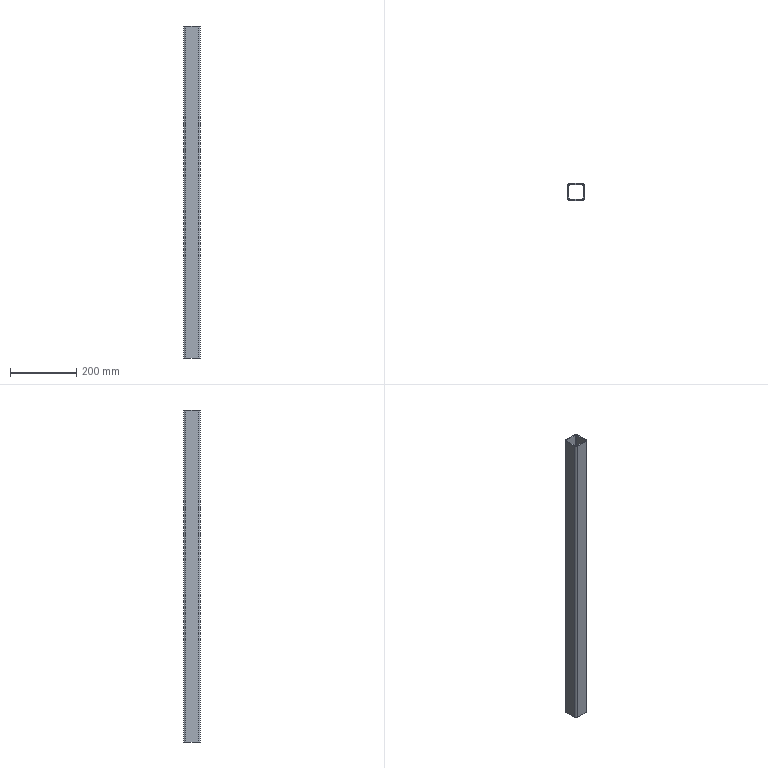Part | SolidWorks | 1 solid | 18 faces | box 50 x 50 x 1000 mm | volume 540823 mm3 | plane 10 | cylinder 8 | commonest cylinder face diameters 6 x4 12 x4
STEP:
#1=CARTESIAN_POINT('',(19.,25.,500.));
#2=VERTEX_POINT('',#1);
#3=CARTESIAN_POINT('',(25.,19.,500.));
#4=VERTEX_POINT('',#3);
#5=CARTESIAN_POINT('',(19.,19.,500.));
#6=DIRECTION('',(0.,0.,-1.));
#7=DIRECTION('',(-1.,0.,0.));
#8=AXIS2_PLACEMENT_3D('',#5,#6,#7);
#9=CIRCLE('',#8,6.);
#10=EDGE_CURVE('',#2,#4,#9,.T.);
#11=ORIENTED_EDGE('',*,*,#10,.T.);
#12=CARTESIAN_POINT('',(25.,19.,-500.));
#13=VERTEX_POINT('',#12);
#14=CARTESIAN_POINT('',(25.,19.,-500.));
#15=DIRECTION('',(0.,0.,1.));
#16=VECTOR('',#15,1000.);
#17=LINE('',#14,#16);
#18=EDGE_CURVE('',#13,#4,#17,.T.);
#19=ORIENTED_EDGE('',*,*,#18,.F.);
#20=CARTESIAN_POINT('',(19.,25.,-500.));
#21=VERTEX_POINT('',#20);
#22=CARTESIAN_POINT('',(19.,19.,-500.));
#23=DIRECTION('',(0.,0.,-1.));
#24=DIRECTION('',(-1.,0.,0.));
#25=AXIS2_PLACEMENT_3D('',#22,#23,#24);
#26=CIRCLE('',#25,6.);
#27=EDGE_CURVE('',#21,#13,#26,.T.);
#28=ORIENTED_EDGE('',*,*,#27,.F.);
#29=CARTESIAN_POINT('',(19.,25.,-500.));
#30=DIRECTION('',(0.,0.,1.));
#31=VECTOR('',#30,1000.);
#32=LINE('',#29,#31);
#33=EDGE_CURVE('',#21,#2,#32,.T.);
#34=ORIENTED_EDGE('',*,*,#33,.T.);
#35=EDGE_LOOP('',(#11,#19,#28,#34));
#36=FACE_OUTER_BOUND('',#35,.T.);
#37=CARTESIAN_POINT('',(19.,19.,-500.));
#38=DIRECTION('',(0.,0.,1.));
#39=DIRECTION('',(1.,0.,0.));
#40=AXIS2_PLACEMENT_3D('',#37,#38,#39);
#41=CYLINDRICAL_SURFACE('',#40,6.);
#42=ADVANCED_FACE('',(#36),#41,.T.);
#43=CARTESIAN_POINT('',(25.,-19.,500.));
#44=VERTEX_POINT('',#43);
#45=CARTESIAN_POINT('',(25.,19.,500.));
#46=DIRECTION('',(0.,-1.,0.));
#47=VECTOR('',#46,1000.);
#48=LINE('',#45,#47);
#49=EDGE_CURVE('',#4,#44,#48,.T.);
#50=ORIENTED_EDGE('',*,*,#49,.T.);
#51=CARTESIAN_POINT('',(25.,-19.,-500.));
#52=VERTEX_POINT('',#51);
#53=CARTESIAN_POINT('',(25.,-19.,-500.));
#54=DIRECTION('',(0.,0.,1.));
#55=VECTOR('',#54,1000.);
#56=LINE('',#53,#55);
#57=EDGE_CURVE('',#52,#44,#56,.T.);
#58=ORIENTED_EDGE('',*,*,#57,.F.);
#59=CARTESIAN_POINT('',(25.,19.,-500.));
#60=DIRECTION('',(0.,-1.,0.));
#61=VECTOR('',#60,1000.);
#62=LINE('',#59,#61);
#63=EDGE_CURVE('',#13,#52,#62,.T.);
#64=ORIENTED_EDGE('',*,*,#63,.F.);
#65=ORIENTED_EDGE('',*,*,#18,.T.);
#66=EDGE_LOOP('',(#50,#58,#64,#65));
#67=FACE_OUTER_BOUND('',#66,.T.);
#68=CARTESIAN_POINT('',(25.,19.,-500.));
#69=DIRECTION('',(-1.,0.,0.));
#70=DIRECTION('',(0.,0.,1.));
#71=AXIS2_PLACEMENT_3D('',#68,#69,#70);
#72=PLANE('',#71);
#73=ADVANCED_FACE('',(#67),#72,.F.);
#74=CARTESIAN_POINT('',(19.,-25.,500.));
#75=VERTEX_POINT('',#74);
#76=CARTESIAN_POINT('',(19.,-19.,500.));
#77=DIRECTION('',(0.,0.,-1.));
#78=DIRECTION('',(-1.,0.,0.));
#79=AXIS2_PLACEMENT_3D('',#76,#77,#78);
#80=CIRCLE('',#79,6.);
#81=EDGE_CURVE('',#44,#75,#80,.T.);
#82=ORIENTED_EDGE('',*,*,#81,.T.);
#83=CARTESIAN_POINT('',(19.,-25.,-500.));
#84=VERTEX_POINT('',#83);
#85=CARTESIAN_POINT('',(19.,-25.,-500.));
#86=DIRECTION('',(0.,0.,1.));
#87=VECTOR('',#86,1000.);
#88=LINE('',#85,#87);
#89=EDGE_CURVE('',#84,#75,#88,.T.);
#90=ORIENTED_EDGE('',*,*,#89,.F.);
#91=CARTESIAN_POINT('',(19.,-19.,-500.));
#92=DIRECTION('',(0.,0.,-1.));
#93=DIRECTION('',(-1.,0.,0.));
#94=AXIS2_PLACEMENT_3D('',#91,#92,#93);
#95=CIRCLE('',#94,6.);
#96=EDGE_CURVE('',#52,#84,#95,.T.);
#97=ORIENTED_EDGE('',*,*,#96,.F.);
#98=ORIENTED_EDGE('',*,*,#57,.T.);
#99=EDGE_LOOP('',(#82,#90,#97,#98));
#100=FACE_OUTER_BOUND('',#99,.T.);
#101=CARTESIAN_POINT('',(19.,-19.,-500.));
#102=DIRECTION('',(0.,0.,1.));
#103=DIRECTION('',(1.,0.,0.));
#104=AXIS2_PLACEMENT_3D('',#101,#102,#103);
#105=CYLINDRICAL_SURFACE('',#104,6.);
#106=ADVANCED_FACE('',(#100),#105,.T.);
#107=CARTESIAN_POINT('',(-19.,-25.,500.));
#108=VERTEX_POINT('',#107);
#109=CARTESIAN_POINT('',(-19.,-25.,500.));
#110=DIRECTION('',(-1.,0.,0.));
#111=VECTOR('',#110,1000.);
#112=LINE('',#109,#111);
#113=EDGE_CURVE('',#75,#108,#112,.T.);
#114=ORIENTED_EDGE('',*,*,#113,.T.);
#115=CARTESIAN_POINT('',(-19.,-25.,-500.));
#116=VERTEX_POINT('',#115);
#117=CARTESIAN_POINT('',(-19.,-25.,-500.));
#118=DIRECTION('',(0.,0.,1.));
#119=VECTOR('',#118,1000.);
#120=LINE('',#117,#119);
#121=EDGE_CURVE('',#116,#108,#120,.T.);
#122=ORIENTED_EDGE('',*,*,#121,.F.);
#123=CARTESIAN_POINT('',(-19.,-25.,-500.));
#124=DIRECTION('',(-1.,0.,0.));
#125=VECTOR('',#124,1000.);
#126=LINE('',#123,#125);
#127=EDGE_CURVE('',#84,#116,#126,.T.);
#128=ORIENTED_EDGE('',*,*,#127,.F.);
#129=ORIENTED_EDGE('',*,*,#89,.T.);
#130=EDGE_LOOP('',(#114,#122,#128,#129));
#131=FACE_OUTER_BOUND('',#130,.T.);
#132=CARTESIAN_POINT('',(-19.,-25.,-500.));
#133=DIRECTION('',(0.,1.,0.));
#134=DIRECTION('',(0.,0.,1.));
#135=AXIS2_PLACEMENT_3D('',#132,#133,#134);
#136=PLANE('',#135);
#137=ADVANCED_FACE('',(#131),#136,.F.);
#138=CARTESIAN_POINT('',(-25.,-19.,500.));
#139=VERTEX_POINT('',#138);
#140=CARTESIAN_POINT('',(-19.,-19.,500.));
#141=DIRECTION('',(0.,0.,-1.));
#142=DIRECTION('',(-1.,0.,0.));
#143=AXIS2_PLACEMENT_3D('',#140,#141,#142);
#144=CIRCLE('',#143,6.);
#145=EDGE_CURVE('',#108,#139,#144,.T.);
#146=ORIENTED_EDGE('',*,*,#145,.T.);
#147=CARTESIAN_POINT('',(-25.,-19.,-500.));
#148=VERTEX_POINT('',#147);
#149=CARTESIAN_POINT('',(-25.,-19.,-500.));
#150=DIRECTION('',(0.,0.,1.));
#151=VECTOR('',#150,1000.);
#152=LINE('',#149,#151);
#153=EDGE_CURVE('',#148,#139,#152,.T.);
#154=ORIENTED_EDGE('',*,*,#153,.F.);
#155=CARTESIAN_POINT('',(-19.,-19.,-500.));
#156=DIRECTION('',(0.,0.,-1.));
#157=DIRECTION('',(-1.,0.,0.));
#158=AXIS2_PLACEMENT_3D('',#155,#156,#157);
#159=CIRCLE('',#158,6.);
#160=EDGE_CURVE('',#116,#148,#159,.T.);
#161=ORIENTED_EDGE('',*,*,#160,.F.);
#162=ORIENTED_EDGE('',*,*,#121,.T.);
#163=EDGE_LOOP('',(#146,#154,#161,#162));
#164=FACE_OUTER_BOUND('',#163,.T.);
#165=CARTESIAN_POINT('',(-19.,-19.,-500.));
#166=DIRECTION('',(0.,0.,1.));
#167=DIRECTION('',(1.,0.,0.));
#168=AXIS2_PLACEMENT_3D('',#165,#166,#167);
#169=CYLINDRICAL_SURFACE('',#168,6.);
#170=ADVANCED_FACE('',(#164),#169,.T.);
#171=CARTESIAN_POINT('',(-25.,19.,500.));
#172=VERTEX_POINT('',#171);
#173=CARTESIAN_POINT('',(-25.,-19.,500.));
#174=DIRECTION('',(0.,1.,0.));
#175=VECTOR('',#174,1000.);
#176=LINE('',#173,#175);
#177=EDGE_CURVE('',#139,#172,#176,.T.);
#178=ORIENTED_EDGE('',*,*,#177,.T.);
#179=CARTESIAN_POINT('',(-25.,19.,-500.));
#180=VERTEX_POINT('',#179);
#181=CARTESIAN_POINT('',(-25.,19.,-500.));
#182=DIRECTION('',(0.,0.,1.));
#183=VECTOR('',#182,1000.);
#184=LINE('',#181,#183);
#185=EDGE_CURVE('',#180,#172,#184,.T.);
#186=ORIENTED_EDGE('',*,*,#185,.F.);
#187=CARTESIAN_POINT('',(-25.,-19.,-500.));
#188=DIRECTION('',(0.,1.,0.));
#189=VECTOR('',#188,1000.);
#190=LINE('',#187,#189);
#191=EDGE_CURVE('',#148,#180,#190,.T.);
#192=ORIENTED_EDGE('',*,*,#191,.F.);
#193=ORIENTED_EDGE('',*,*,#153,.T.);
#194=EDGE_LOOP('',(#178,#186,#192,#193));
#195=FACE_OUTER_BOUND('',#194,.T.);
#196=CARTESIAN_POINT('',(-25.,-19.,-500.));
#197=DIRECTION('',(1.,0.,0.));
#198=DIRECTION('',(0.,0.,-1.));
#199=AXIS2_PLACEMENT_3D('',#196,#197,#198);
#200=PLANE('',#199);
#201=ADVANCED_FACE('',(#195),#200,.F.);
#202=CARTESIAN_POINT('',(-19.,25.,500.));
#203=VERTEX_POINT('',#202);
#204=CARTESIAN_POINT('',(-19.,19.,500.));
#205=DIRECTION('',(0.,0.,-1.));
#206=DIRECTION('',(-1.,0.,0.));
#207=AXIS2_PLACEMENT_3D('',#204,#205,#206);
#208=CIRCLE('',#207,6.);
#209=EDGE_CURVE('',#172,#203,#208,.T.);
#210=ORIENTED_EDGE('',*,*,#209,.T.);
#211=CARTESIAN_POINT('',(-19.,25.,-500.));
#212=VERTEX_POINT('',#211);
#213=CARTESIAN_POINT('',(-19.,25.,-500.));
#214=DIRECTION('',(0.,0.,1.));
#215=VECTOR('',#214,1000.);
#216=LINE('',#213,#215);
#217=EDGE_CURVE('',#212,#203,#216,.T.);
#218=ORIENTED_EDGE('',*,*,#217,.F.);
#219=CARTESIAN_POINT('',(-19.,19.,-500.));
#220=DIRECTION('',(0.,0.,-1.));
#221=DIRECTION('',(-1.,0.,0.));
#222=AXIS2_PLACEMENT_3D('',#219,#220,#221);
#223=CIRCLE('',#222,6.);
#224=EDGE_CURVE('',#180,#212,#223,.T.);
#225=ORIENTED_EDGE('',*,*,#224,.F.);
#226=ORIENTED_EDGE('',*,*,#185,.T.);
#227=EDGE_LOOP('',(#210,#218,#225,#226));
#228=FACE_OUTER_BOUND('',#227,.T.);
#229=CARTESIAN_POINT('',(-19.,19.,-500.));
#230=DIRECTION('',(0.,0.,1.));
#231=DIRECTION('',(1.,0.,0.));
#232=AXIS2_PLACEMENT_3D('',#229,#230,#231);
#233=CYLINDRICAL_SURFACE('',#232,6.);
#234=ADVANCED_FACE('',(#228),#233,.T.);
#235=CARTESIAN_POINT('',(22.,-19.,500.));
#236=VERTEX_POINT('',#235);
#237=CARTESIAN_POINT('',(19.,-22.,500.));
#238=VERTEX_POINT('',#237);
#239=CARTESIAN_POINT('',(19.,-19.,500.));
#240=DIRECTION('',(0.,0.,-1.));
#241=DIRECTION('',(-1.,0.,0.));
#242=AXIS2_PLACEMENT_3D('',#239,#240,#241);
#243=CIRCLE('',#242,3.);
#244=EDGE_CURVE('',#236,#238,#243,.T.);
#245=ORIENTED_EDGE('',*,*,#244,.F.);
#246=CARTESIAN_POINT('',(22.,-19.,-500.));
#247=VERTEX_POINT('',#246);
#248=CARTESIAN_POINT('',(22.,-19.,-500.));
#249=DIRECTION('',(0.,0.,1.));
#250=VECTOR('',#249,1000.);
#251=LINE('',#248,#250);
#252=EDGE_CURVE('',#247,#236,#251,.T.);
#253=ORIENTED_EDGE('',*,*,#252,.F.);
#254=CARTESIAN_POINT('',(19.,-22.,-500.));
#255=VERTEX_POINT('',#254);
#256=CARTESIAN_POINT('',(19.,-19.,-500.));
#257=DIRECTION('',(0.,0.,-1.));
#258=DIRECTION('',(-1.,0.,0.));
#259=AXIS2_PLACEMENT_3D('',#256,#257,#258);
#260=CIRCLE('',#259,3.);
#261=EDGE_CURVE('',#247,#255,#260,.T.);
#262=ORIENTED_EDGE('',*,*,#261,.T.);
#263=CARTESIAN_POINT('',(19.,-22.,-500.));
#264=DIRECTION('',(0.,0.,1.));
#265=VECTOR('',#264,1000.);
#266=LINE('',#263,#265);
#267=EDGE_CURVE('',#255,#238,#266,.T.);
#268=ORIENTED_EDGE('',*,*,#267,.T.);
#269=EDGE_LOOP('',(#245,#253,#262,#268));
#270=FACE_OUTER_BOUND('',#269,.T.);
#271=CARTESIAN_POINT('',(19.,-19.,-500.));
#272=DIRECTION('',(0.,0.,1.));
#273=DIRECTION('',(1.,0.,0.));
#274=AXIS2_PLACEMENT_3D('',#271,#272,#273);
#275=CYLINDRICAL_SURFACE('',#274,3.);
#276=ADVANCED_FACE('',(#270),#275,.F.);
#277=CARTESIAN_POINT('',(22.,19.,500.));
#278=VERTEX_POINT('',#277);
#279=CARTESIAN_POINT('',(22.,19.,500.));
#280=DIRECTION('',(0.,-1.,0.));
#281=VECTOR('',#280,1000.);
#282=LINE('',#279,#281);
#283=EDGE_CURVE('',#278,#236,#282,.T.);
#284=ORIENTED_EDGE('',*,*,#283,.F.);
#285=CARTESIAN_POINT('',(22.,19.,-500.));
#286=VERTEX_POINT('',#285);
#287=CARTESIAN_POINT('',(22.,19.,-500.));
#288=DIRECTION('',(0.,0.,1.));
#289=VECTOR('',#288,1000.);
#290=LINE('',#287,#289);
#291=EDGE_CURVE('',#286,#278,#290,.T.);
#292=ORIENTED_EDGE('',*,*,#291,.F.);
#293=CARTESIAN_POINT('',(22.,19.,-500.));
#294=DIRECTION('',(0.,-1.,0.));
#295=VECTOR('',#294,1000.);
#296=LINE('',#293,#295);
#297=EDGE_CURVE('',#286,#247,#296,.T.);
#298=ORIENTED_EDGE('',*,*,#297,.T.);
#299=ORIENTED_EDGE('',*,*,#252,.T.);
#300=EDGE_LOOP('',(#284,#292,#298,#299));
#301=FACE_OUTER_BOUND('',#300,.T.);
#302=CARTESIAN_POINT('',(22.,19.,-500.));
#303=DIRECTION('',(-1.,0.,0.));
#304=DIRECTION('',(0.,0.,1.));
#305=AXIS2_PLACEMENT_3D('',#302,#303,#304);
#306=PLANE('',#305);
#307=ADVANCED_FACE('',(#301),#306,.T.);
#308=CARTESIAN_POINT('',(19.,22.,500.));
#309=VERTEX_POINT('',#308);
#310=CARTESIAN_POINT('',(19.,19.,500.));
#311=DIRECTION('',(0.,0.,-1.));
#312=DIRECTION('',(-1.,0.,0.));
#313=AXIS2_PLACEMENT_3D('',#310,#311,#312);
#314=CIRCLE('',#313,3.);
#315=EDGE_CURVE('',#309,#278,#314,.T.);
#316=ORIENTED_EDGE('',*,*,#315,.F.);
#317=CARTESIAN_POINT('',(19.,22.,-500.));
#318=VERTEX_POINT('',#317);
#319=CARTESIAN_POINT('',(19.,22.,-500.));
#320=DIRECTION('',(0.,0.,1.));
#321=VECTOR('',#320,1000.);
#322=LINE('',#319,#321);
#323=EDGE_CURVE('',#318,#309,#322,.T.);
#324=ORIENTED_EDGE('',*,*,#323,.F.);
#325=CARTESIAN_POINT('',(19.,19.,-500.));
#326=DIRECTION('',(0.,0.,-1.));
#327=DIRECTION('',(-1.,0.,0.));
#328=AXIS2_PLACEMENT_3D('',#325,#326,#327);
#329=CIRCLE('',#328,3.);
#330=EDGE_CURVE('',#318,#286,#329,.T.);
#331=ORIENTED_EDGE('',*,*,#330,.T.);
#332=ORIENTED_EDGE('',*,*,#291,.T.);
#333=EDGE_LOOP('',(#316,#324,#331,#332));
#334=FACE_OUTER_BOUND('',#333,.T.);
#335=CARTESIAN_POINT('',(19.,19.,-500.));
#336=DIRECTION('',(0.,0.,1.));
#337=DIRECTION('',(1.,0.,0.));
#338=AXIS2_PLACEMENT_3D('',#335,#336,#337);
#339=CYLINDRICAL_SURFACE('',#338,3.);
#340=ADVANCED_FACE('',(#334),#339,.F.);
#341=CARTESIAN_POINT('',(-19.,22.,500.));
#342=VERTEX_POINT('',#341);
#343=CARTESIAN_POINT('',(19.,22.,500.));
#344=DIRECTION('',(1.,0.,0.));
#345=VECTOR('',#344,1000.);
#346=LINE('',#343,#345);
#347=EDGE_CURVE('',#342,#309,#346,.T.);
#348=ORIENTED_EDGE('',*,*,#347,.F.);
#349=CARTESIAN_POINT('',(-19.,22.,-500.));
#350=VERTEX_POINT('',#349);
#351=CARTESIAN_POINT('',(-19.,22.,-500.));
#352=DIRECTION('',(0.,0.,1.));
#353=VECTOR('',#352,1000.);
#354=LINE('',#351,#353);
#355=EDGE_CURVE('',#350,#342,#354,.T.);
#356=ORIENTED_EDGE('',*,*,#355,.F.);
#357=CARTESIAN_POINT('',(19.,22.,-500.));
#358=DIRECTION('',(1.,0.,0.));
#359=VECTOR('',#358,1000.);
#360=LINE('',#357,#359);
#361=EDGE_CURVE('',#350,#318,#360,.T.);
#362=ORIENTED_EDGE('',*,*,#361,.T.);
#363=ORIENTED_EDGE('',*,*,#323,.T.);
#364=EDGE_LOOP('',(#348,#356,#362,#363));
#365=FACE_OUTER_BOUND('',#364,.T.);
#366=CARTESIAN_POINT('',(19.,22.,-500.));
#367=DIRECTION('',(0.,-1.,0.));
#368=DIRECTION('',(0.,0.,-1.));
#369=AXIS2_PLACEMENT_3D('',#366,#367,#368);
#370=PLANE('',#369);
#371=ADVANCED_FACE('',(#365),#370,.T.);
#372=CARTESIAN_POINT('',(-22.,19.,500.));
#373=VERTEX_POINT('',#372);
#374=CARTESIAN_POINT('',(-19.,19.,500.));
#375=DIRECTION('',(0.,0.,-1.));
#376=DIRECTION('',(-1.,0.,0.));
#377=AXIS2_PLACEMENT_3D('',#374,#375,#376);
#378=CIRCLE('',#377,3.);
#379=EDGE_CURVE('',#373,#342,#378,.T.);
#380=ORIENTED_EDGE('',*,*,#379,.F.);
#381=CARTESIAN_POINT('',(-22.,19.,-500.));
#382=VERTEX_POINT('',#381);
#383=CARTESIAN_POINT('',(-22.,19.,-500.));
#384=DIRECTION('',(0.,0.,1.));
#385=VECTOR('',#384,1000.);
#386=LINE('',#383,#385);
#387=EDGE_CURVE('',#382,#373,#386,.T.);
#388=ORIENTED_EDGE('',*,*,#387,.F.);
#389=CARTESIAN_POINT('',(-19.,19.,-500.));
#390=DIRECTION('',(0.,0.,-1.));
#391=DIRECTION('',(-1.,0.,0.));
#392=AXIS2_PLACEMENT_3D('',#389,#390,#391);
#393=CIRCLE('',#392,3.);
#394=EDGE_CURVE('',#382,#350,#393,.T.);
#395=ORIENTED_EDGE('',*,*,#394,.T.);
#396=ORIENTED_EDGE('',*,*,#355,.T.);
#397=EDGE_LOOP('',(#380,#388,#395,#396));
#398=FACE_OUTER_BOUND('',#397,.T.);
#399=CARTESIAN_POINT('',(-19.,19.,-500.));
#400=DIRECTION('',(0.,0.,1.));
#401=DIRECTION('',(1.,0.,0.));
#402=AXIS2_PLACEMENT_3D('',#399,#400,#401);
#403=CYLINDRICAL_SURFACE('',#402,3.);
#404=ADVANCED_FACE('',(#398),#403,.F.);
#405=CARTESIAN_POINT('',(-22.,-19.,500.));
#406=VERTEX_POINT('',#405);
#407=CARTESIAN_POINT('',(-22.,-19.,500.));
#408=DIRECTION('',(0.,1.,0.));
#409=VECTOR('',#408,1000.);
#410=LINE('',#407,#409);
#411=EDGE_CURVE('',#406,#373,#410,.T.);
#412=ORIENTED_EDGE('',*,*,#411,.F.);
#413=CARTESIAN_POINT('',(-22.,-19.,-500.));
#414=VERTEX_POINT('',#413);
#415=CARTESIAN_POINT('',(-22.,-19.,-500.));
#416=DIRECTION('',(0.,0.,1.));
#417=VECTOR('',#416,1000.);
#418=LINE('',#415,#417);
#419=EDGE_CURVE('',#414,#406,#418,.T.);
#420=ORIENTED_EDGE('',*,*,#419,.F.);
#421=CARTESIAN_POINT('',(-22.,-19.,-500.));
#422=DIRECTION('',(0.,1.,0.));
#423=VECTOR('',#422,1000.);
#424=LINE('',#421,#423);
#425=EDGE_CURVE('',#414,#382,#424,.T.);
#426=ORIENTED_EDGE('',*,*,#425,.T.);
#427=ORIENTED_EDGE('',*,*,#387,.T.);
#428=EDGE_LOOP('',(#412,#420,#426,#427));
#429=FACE_OUTER_BOUND('',#428,.T.);
#430=CARTESIAN_POINT('',(-22.,-19.,-500.));
#431=DIRECTION('',(1.,0.,0.));
#432=DIRECTION('',(0.,0.,-1.));
#433=AXIS2_PLACEMENT_3D('',#430,#431,#432);
#434=PLANE('',#433);
#435=ADVANCED_FACE('',(#429),#434,.T.);
#436=CARTESIAN_POINT('',(-19.,-22.,500.));
#437=VERTEX_POINT('',#436);
#438=CARTESIAN_POINT('',(-19.,-19.,500.));
#439=DIRECTION('',(0.,0.,-1.));
#440=DIRECTION('',(-1.,0.,0.));
#441=AXIS2_PLACEMENT_3D('',#438,#439,#440);
#442=CIRCLE('',#441,3.);
#443=EDGE_CURVE('',#437,#406,#442,.T.);
#444=ORIENTED_EDGE('',*,*,#443,.F.);
#445=CARTESIAN_POINT('',(-19.,-22.,-500.));
#446=VERTEX_POINT('',#445);
#447=CARTESIAN_POINT('',(-19.,-22.,-500.));
#448=DIRECTION('',(0.,0.,1.));
#449=VECTOR('',#448,1000.);
#450=LINE('',#447,#449);
#451=EDGE_CURVE('',#446,#437,#450,.T.);
#452=ORIENTED_EDGE('',*,*,#451,.F.);
#453=CARTESIAN_POINT('',(-19.,-19.,-500.));
#454=DIRECTION('',(0.,0.,-1.));
#455=DIRECTION('',(-1.,0.,0.));
#456=AXIS2_PLACEMENT_3D('',#453,#454,#455);
#457=CIRCLE('',#456,3.);
#458=EDGE_CURVE('',#446,#414,#457,.T.);
#459=ORIENTED_EDGE('',*,*,#458,.T.);
#460=ORIENTED_EDGE('',*,*,#419,.T.);
#461=EDGE_LOOP('',(#444,#452,#459,#460));
#462=FACE_OUTER_BOUND('',#461,.T.);
#463=CARTESIAN_POINT('',(-19.,-19.,-500.));
#464=DIRECTION('',(0.,0.,1.));
#465=DIRECTION('',(1.,0.,0.));
#466=AXIS2_PLACEMENT_3D('',#463,#464,#465);
#467=CYLINDRICAL_SURFACE('',#466,3.);
#468=ADVANCED_FACE('',(#462),#467,.F.);
#469=CARTESIAN_POINT('',(-19.,-22.,500.));
#470=DIRECTION('',(-1.,0.,0.));
#471=VECTOR('',#470,1000.);
#472=LINE('',#469,#471);
#473=EDGE_CURVE('',#238,#437,#472,.T.);
#474=ORIENTED_EDGE('',*,*,#473,.F.);
#475=ORIENTED_EDGE('',*,*,#267,.F.);
#476=CARTESIAN_POINT('',(-19.,-22.,-500.));
#477=DIRECTION('',(-1.,0.,0.));
#478=VECTOR('',#477,1000.);
#479=LINE('',#476,#478);
#480=EDGE_CURVE('',#255,#446,#479,.T.);
#481=ORIENTED_EDGE('',*,*,#480,.T.);
#482=ORIENTED_EDGE('',*,*,#451,.T.);
#483=EDGE_LOOP('',(#474,#475,#481,#482));
#484=FACE_OUTER_BOUND('',#483,.T.);
#485=CARTESIAN_POINT('',(-19.,-22.,-500.));
#486=DIRECTION('',(0.,1.,0.));
#487=DIRECTION('',(0.,0.,1.));
#488=AXIS2_PLACEMENT_3D('',#485,#486,#487);
#489=PLANE('',#488);
#490=ADVANCED_FACE('',(#484),#489,.T.);
#491=CARTESIAN_POINT('',(19.,25.,500.));
#492=DIRECTION('',(1.,0.,0.));
#493=VECTOR('',#492,1000.);
#494=LINE('',#491,#493);
#495=EDGE_CURVE('',#203,#2,#494,.T.);
#496=ORIENTED_EDGE('',*,*,#495,.T.);
#497=ORIENTED_EDGE('',*,*,#33,.F.);
#498=CARTESIAN_POINT('',(19.,25.,-500.));
#499=DIRECTION('',(1.,0.,0.));
#500=VECTOR('',#499,1000.);
#501=LINE('',#498,#500);
#502=EDGE_CURVE('',#212,#21,#501,.T.);
#503=ORIENTED_EDGE('',*,*,#502,.F.);
#504=ORIENTED_EDGE('',*,*,#217,.T.);
#505=EDGE_LOOP('',(#496,#497,#503,#504));
#506=FACE_OUTER_BOUND('',#505,.T.);
#507=CARTESIAN_POINT('',(19.,25.,-500.));
#508=DIRECTION('',(0.,-1.,0.));
#509=DIRECTION('',(0.,0.,-1.));
#510=AXIS2_PLACEMENT_3D('',#507,#508,#509);
#511=PLANE('',#510);
#512=ADVANCED_FACE('',(#506),#511,.F.);
#513=ORIENTED_EDGE('',*,*,#261,.F.);
#514=ORIENTED_EDGE('',*,*,#297,.F.);
#515=ORIENTED_EDGE('',*,*,#330,.F.);
#516=ORIENTED_EDGE('',*,*,#361,.F.);
#517=ORIENTED_EDGE('',*,*,#394,.F.);
#518=ORIENTED_EDGE('',*,*,#425,.F.);
#519=ORIENTED_EDGE('',*,*,#458,.F.);
#520=ORIENTED_EDGE('',*,*,#480,.F.);
#521=EDGE_LOOP('',(#513,#514,#515,#516,#517,#518,#519,#520));
#522=FACE_BOUND('',#521,.T.);
#523=ORIENTED_EDGE('',*,*,#27,.T.);
#524=ORIENTED_EDGE('',*,*,#63,.T.);
#525=ORIENTED_EDGE('',*,*,#96,.T.);
#526=ORIENTED_EDGE('',*,*,#127,.T.);
#527=ORIENTED_EDGE('',*,*,#160,.T.);
#528=ORIENTED_EDGE('',*,*,#191,.T.);
#529=ORIENTED_EDGE('',*,*,#224,.T.);
#530=ORIENTED_EDGE('',*,*,#502,.T.);
#531=EDGE_LOOP('',(#523,#524,#525,#526,#527,#528,#529,#530));
#532=FACE_OUTER_BOUND('',#531,.T.);
#533=CARTESIAN_POINT('',(19.,19.,-500.));
#534=DIRECTION('',(0.,0.,-1.));
#535=DIRECTION('',(-1.,0.,0.));
#536=AXIS2_PLACEMENT_3D('',#533,#534,#535);
#537=PLANE('',#536);
#538=ADVANCED_FACE('',(#522,#532),#537,.T.);
#539=ORIENTED_EDGE('',*,*,#244,.T.);
#540=ORIENTED_EDGE('',*,*,#473,.T.);
#541=ORIENTED_EDGE('',*,*,#443,.T.);
#542=ORIENTED_EDGE('',*,*,#411,.T.);
#543=ORIENTED_EDGE('',*,*,#379,.T.);
#544=ORIENTED_EDGE('',*,*,#347,.T.);
#545=ORIENTED_EDGE('',*,*,#315,.T.);
#546=ORIENTED_EDGE('',*,*,#283,.T.);
#547=EDGE_LOOP('',(#539,#540,#541,#542,#543,#544,#545,#546));
#548=FACE_BOUND('',#547,.T.);
#549=ORIENTED_EDGE('',*,*,#10,.F.);
#550=ORIENTED_EDGE('',*,*,#495,.F.);
#551=ORIENTED_EDGE('',*,*,#209,.F.);
#552=ORIENTED_EDGE('',*,*,#177,.F.);
#553=ORIENTED_EDGE('',*,*,#145,.F.);
#554=ORIENTED_EDGE('',*,*,#113,.F.);
#555=ORIENTED_EDGE('',*,*,#81,.F.);
#556=ORIENTED_EDGE('',*,*,#49,.F.);
#557=EDGE_LOOP('',(#549,#550,#551,#552,#553,#554,#555,#556));
#558=FACE_OUTER_BOUND('',#557,.T.);
#559=CARTESIAN_POINT('',(19.,19.,500.));
#560=DIRECTION('',(0.,0.,-1.));
#561=DIRECTION('',(-1.,0.,0.));
#562=AXIS2_PLACEMENT_3D('',#559,#560,#561);
#563=PLANE('',#562);
#564=ADVANCED_FACE('',(#548,#558),#563,.F.);
#565=CLOSED_SHELL('',(#42,#73,#106,#137,#170,#201,#234,#276,#307,#340,#371,#404,#435,#468,#490,#512,#538,#564));
#566=MANIFOLD_SOLID_BREP('',#565);
#567=CARTESIAN_POINT('',(0.,0.,0.));
#568=DIRECTION('',(0.,0.,1.));
#569=DIRECTION('',(1.,0.,0.));
#570=AXIS2_PLACEMENT_3D('',#567,#568,#569);
#571=(LENGTH_UNIT()NAMED_UNIT(*)SI_UNIT(.MILLI.,.METRE.));
#572=UNCERTAINTY_MEASURE_WITH_UNIT(LENGTH_MEASURE(0.00001),#571,'','');
#573=(NAMED_UNIT(*)PLANE_ANGLE_UNIT()SI_UNIT($,.RADIAN.));
#574=(NAMED_UNIT(*)SI_UNIT($,.STERADIAN.)SOLID_ANGLE_UNIT());
#575=(GEOMETRIC_REPRESENTATION_CONTEXT(3)GLOBAL_UNCERTAINTY_ASSIGNED_CONTEXT((#572))GLOBAL_UNIT_ASSIGNED_CONTEXT((#571,#573,#574))REPRESENTATION_CONTEXT('',''));
#576=ADVANCED_BREP_SHAPE_REPRESENTATION('',(#566,#570),#575);